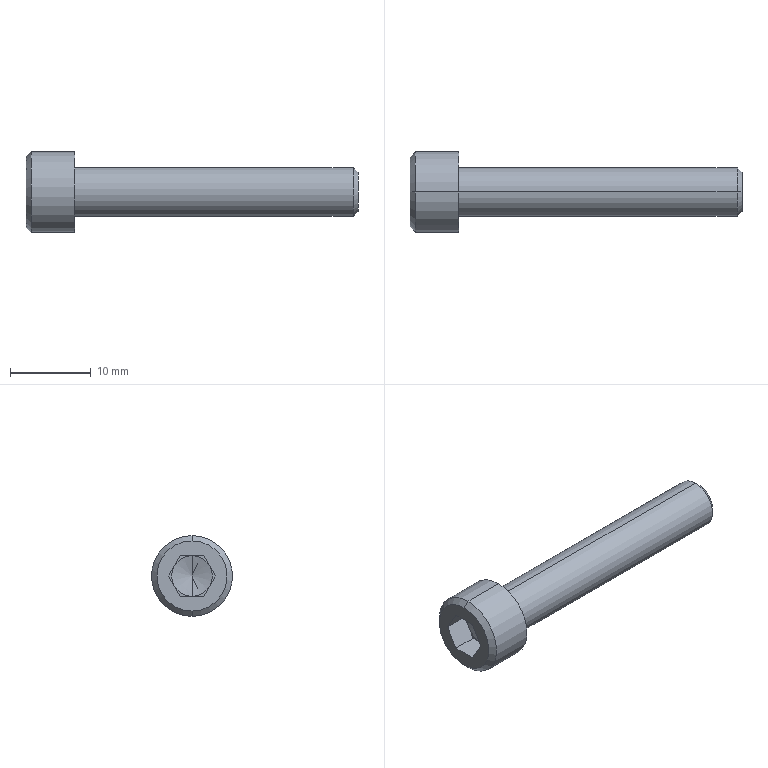Part | STEP file | CB6-35 | 1 solid | 25 faces | box 41 x 10 x 10 mm | volume 1382 mm3 | plane 15 | cone 6 | cylinder 4 | commonest cylinder face diameters 6 x2 10 x2